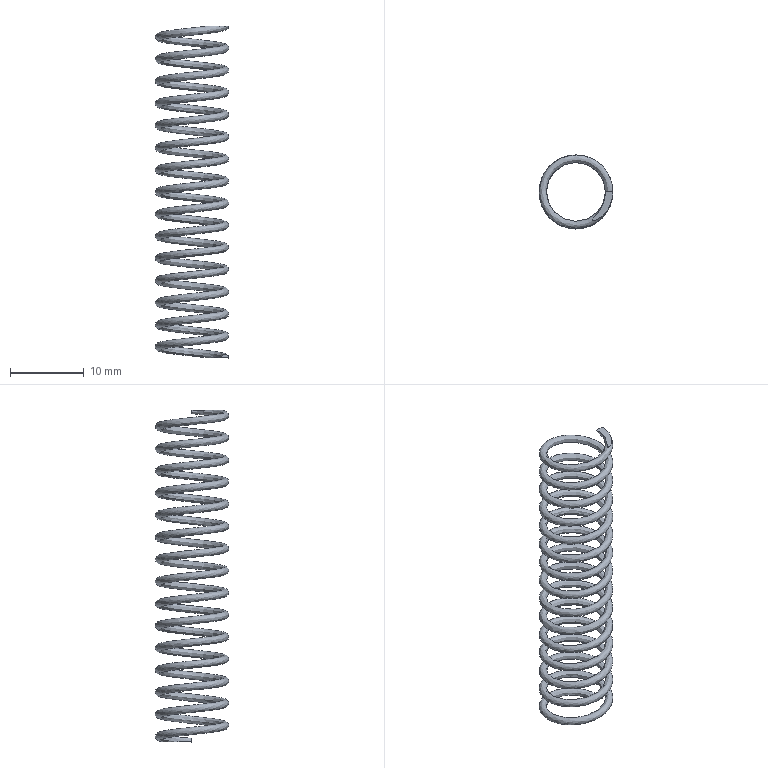Part | STEP file | gslz 2016.10.28-6_id330_x_t | 1 solid | 5 faces | box 9.997 x 9.994 x 45 mm | volume 331.132 mm3 | plane 4 | spline 1